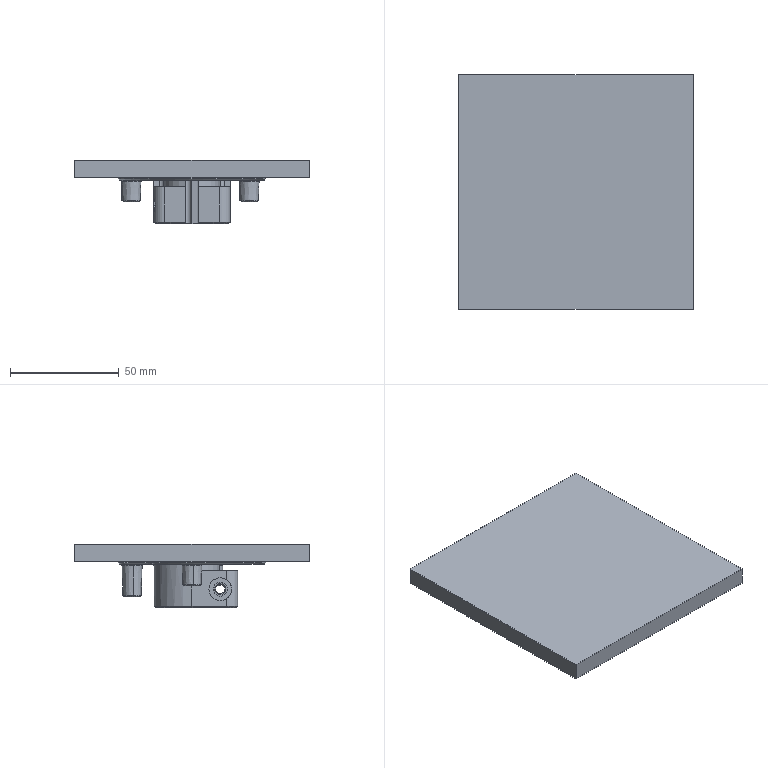NC program | NX | posted with a generic post | part box 108 x 108 x 29 mm
Lines 1354 to 2334 of 23883:
(CAVITY_MILL_COPY , TOOL : D6JING)
N2694 T16 M6
N2696 G54
N2698 G17 G0 G90 X1.893 Y-24.936 S9500 M3
N2700 G43 Z30. H16
N2702 Z1.115
N2704 G94 G1 Z-0.385 F1000.
N2706 X1.909 Y-24.321
N2708 G3 X1.432 Y-23.442 R1.
N2710 G2 X0. Y-20.885 R3. F1500.
N2712 G1 Y-20.5
N2714 Y-20.885
N2716 G2 X-1.432 Y-23.442 R3.
N2718 G3 X-1.909 Y-24.321 R1.
N2720 G1 X-1.893 Y-24.936
N2722 Z1.115
N2724 G0 Z30.
N2726 X1.893 Y-25.052
N2728 Z0.731
N2730 G1 Z-0.769 F1000.
N2732 X1.909 Y-24.437
N2734 G3 X1.432 Y-23.558 R1.
N2736 G2 X0. Y-21. R3. F1500.
N2738 G1 Y-20.5
N2740 Y-21.
N2742 G2 X-1.432 Y-23.558 R3.
N2744 G3 X-1.91 Y-24.437 R1.
N2746 G1 X-1.893 Y-25.052
N2748 Z0.731
N2750 G0 Z30.
N2752 X1.893
N2754 Z0.346
N2756 G1 Z-1.154 F1000.
N2758 X1.909 Y-24.437
N2760 G3 X1.432 Y-23.558 R1.
N2762 G2 X0. Y-21. R3. F1500.
N2764 G1 Y-20.5
N2766 Y-21.
N2768 G2 X-1.432 Y-23.558 R3.
N2770 G3 X-1.91 Y-24.437 R1.
N2772 G1 X-1.893 Y-25.052
N2774 Z0.346
N2776 G0 X1.893 Z-0.038
N2778 G1 Z-1.538 F1000.
N2780 X1.909 Y-24.437
N2782 G3 X1.432 Y-23.558 R1.
N2784 G2 X0. Y-21. R3. F1500.
N2786 G1 Y-20.5
N2788 Y-21.
N2790 G2 X-1.432 Y-23.558 R3.
N2792 G3 X-1.91 Y-24.437 R1.
N2794 G1 X-1.893 Y-25.052
N2796 Z-0.038
N2798 G0 X1.893 Z-0.423
N2800 G1 Z-1.923 F1000.
N2802 X1.909 Y-24.437
N2804 G3 X1.432 Y-23.558 R1.
N2806 G2 X0. Y-21. R3. F1500.
N2808 G1 Y-20.5
N2810 Y-21.
N2812 G2 X-1.432 Y-23.558 R3.
N2814 G3 X-1.91 Y-24.437 R1.
N2816 G1 X-1.893 Y-25.052
N2818 Z-0.423
N2820 G0 X1.893 Z-0.808
N2822 G1 Z-2.308 F1000.
N2824 X1.909 Y-24.437
N2826 G3 X1.432 Y-23.558 R1.
N2828 G2 X0. Y-21. R3. F1500.
N2830 G1 Y-20.5
N2832 Y-21.
N2834 G2 X-1.432 Y-23.558 R3.
N2836 G3 X-1.91 Y-24.437 R1.
N2838 G1 X-1.893 Y-25.052
N2840 Z-0.808
N2842 G0 X1.893 Z-1.192
N2844 G1 Z-2.692 F1000.
N2846 X1.909 Y-24.437
N2848 G3 X1.432 Y-23.558 R1.
N2850 G2 X0. Y-21. R3. F1500.
N2852 G1 Y-20.5
N2854 Y-21.
N2856 G2 X-1.432 Y-23.558 R3.
N2858 G3 X-1.91 Y-24.437 R1.
N2860 G1 X-1.893 Y-25.052
N2862 Z-1.192
N2864 G0 X1.893 Z-1.577
N2866 G1 Z-3.077 F1000.
N2868 X1.909 Y-24.437
N2870 G3 X1.432 Y-23.558 R1.
N2872 G2 X0. Y-21. R3. F1500.
N2874 G1 Y-20.5
N2876 Y-21.
N2878 G2 X-1.432 Y-23.558 R3.
N2880 G3 X-1.91 Y-24.437 R1.
N2882 G1 X-1.893 Y-25.052
N2884 Z-1.577
N2886 G0 X1.893 Z-1.962
N2888 G1 Z-3.462 F1000.
N2890 X1.909 Y-24.437
N2892 G3 X1.432 Y-23.558 R1.
N2894 G2 X0. Y-21. R3. F1500.
N2896 G1 Y-20.5
N2898 Y-21.
N2900 G2 X-1.432 Y-23.558 R3.
N2902 G3 X-1.91 Y-24.437 R1.
N2904 G1 X-1.893 Y-25.052
N2906 Z-1.962
N2908 G0 X1.893 Z-2.346
N2910 G1 Z-3.846 F1000.
N2912 X1.909 Y-24.437
N2914 G3 X1.432 Y-23.558 R1.
N2916 G2 X0. Y-21. R3. F1500.
N2918 G1 Y-20.5
N2920 Y-21.
N2922 G2 X-1.432 Y-23.558 R3.
N2924 G3 X-1.91 Y-24.437 R1.
N2926 G1 X-1.893 Y-25.052
N2928 Z-2.346
N2930 G0 X1.893 Z-2.731
N2932 G1 Z-4.231 F1000.
N2934 X1.909 Y-24.437
N2936 G3 X1.432 Y-23.558 R1.
N2938 G2 X0. Y-21. R3. F1500.
N2940 G1 Y-20.5
N2942 Y-21.
N2944 G2 X-1.432 Y-23.558 R3.
N2946 G3 X-1.91 Y-24.437 R1.
N2948 G1 X-1.893 Y-25.052
N2950 Z-2.731
N2952 G0 X1.893 Z-3.115
N2954 G1 Z-4.615 F1000.
N2956 X1.909 Y-24.437
N2958 G3 X1.432 Y-23.558 R1.
N2960 G2 X0. Y-21. R3. F1500.
N2962 G1 Y-20.501
N2964 Y-21.
N2966 G2 X-1.432 Y-23.558 R3.
N2968 G3 X-1.91 Y-24.437 R1.
N2970 G1 X-1.893 Y-25.052
N2972 Z-3.115
N2974 G0 X1.893 Z-3.5
N2976 G1 Z-5. F1000.
N2978 X1.909 Y-24.437
N2980 G3 X1.432 Y-23.558 R1.
N2982 G2 X0. Y-21. R3. F1500.
N2984 G1 Y-20.501
N2986 Y-21.
N2988 G2 X-1.432 Y-23.558 R3.
N2990 G3 X-1.91 Y-24.437 R1.
N2992 G1 X-1.893 Y-25.052
N2994 Z-3.5
N2996 G0 X1.893 Z-3.885
N2998 G1 Z-5.385 F1000.
N3000 X1.909 Y-24.437
N3002 G3 X1.432 Y-23.558 R1.
N3004 G2 X0. Y-21. R3. F1500.
N3006 G1 Y-20.501
N3008 Y-21.
N3010 G2 X-1.432 Y-23.558 R3.
N3012 G3 X-1.91 Y-24.437 R1.
N3014 G1 X-1.893 Y-25.052
N3016 Z-3.885
N3018 G0 X1.893 Z-4.269
N3020 G1 Z-5.769 F1000.
N3022 X1.909 Y-24.437
N3024 G3 X1.432 Y-23.558 R1.
N3026 G2 X0. Y-21. R3. F1500.
N3028 G1 Y-20.501
N3030 Y-21.
N3032 G2 X-1.432 Y-23.558 R3.
N3034 G3 X-1.91 Y-24.437 R1.
N3036 G1 X-1.893 Y-25.052
N3038 Z-4.269
N3040 G0 X1.893 Z-4.654
N3042 G1 Z-6.154 F1000.
N3044 X1.909 Y-24.437
N3046 G3 X1.432 Y-23.558 R1.
N3048 G2 X0. Y-21. R3. F1500.
N3050 G1 Y-20.501
N3052 Y-21.
N3054 G2 X-1.432 Y-23.558 R3.
N3056 G3 X-1.91 Y-24.437 R1.
N3058 G1 X-1.893 Y-25.052
N3060 Z-4.654
N3062 G0 X1.893 Z-5.038
N3064 G1 Z-6.538 F1000.
N3066 X1.909 Y-24.437
N3068 G3 X1.432 Y-23.558 R1.
N3070 G2 X0. Y-21. R3. F1500.
N3072 G1 Y-20.501
N3074 Y-21.
N3076 G2 X-1.432 Y-23.558 R3.
N3078 G3 X-1.91 Y-24.437 R1.
N3080 G1 X-1.893 Y-25.052
N3082 Z-5.038
N3084 G0 X1.893 Z-5.423
N3086 G1 Z-6.923 F1000.
N3088 X1.909 Y-24.437
N3090 G3 X1.432 Y-23.558 R1.
N3092 G2 X0. Y-21. R3. F1500.
N3094 G1 Y-20.501
N3096 Y-21.
N3098 G2 X-1.432 Y-23.558 R3.
N3100 G3 X-1.91 Y-24.437 R1.
N3102 G1 X-1.893 Y-25.052
N3104 Z-5.423
N3106 G0 X1.893 Z-5.808
N3108 G1 Z-7.308 F1000.
N3110 X1.909 Y-24.437
N3112 G3 X1.432 Y-23.558 R1.
N3114 G2 X0. Y-21. R3. F1500.
N3116 G1 Y-20.501
N3118 Y-21.
N3120 G2 X-1.432 Y-23.558 R3.
N3122 G3 X-1.91 Y-24.437 R1.
N3124 G1 X-1.893 Y-25.052
N3126 Z-5.808
N3128 G0 X1.893 Z-6.192
N3130 G1 Z-7.692 F1000.
N3132 X1.909 Y-24.437
N3134 G3 X1.432 Y-23.558 R1.
N3136 G2 X0. Y-21. R3. F1500.
N3138 G1 Y-20.501
N3140 Y-21.
N3142 G2 X-1.432 Y-23.558 R3.
N3144 G3 X-1.91 Y-24.437 R1.
N3146 G1 X-1.893 Y-25.052
N3148 Z-6.192
N3150 G0 X1.893 Z-6.577
N3152 G1 Z-8.077 F1000.
N3154 X1.909 Y-24.437
N3156 G3 X1.432 Y-23.558 R1.
N3158 G2 X0. Y-21. R3. F1500.
N3160 G1 Y-20.501
N3162 Y-21.
N3164 G2 X-1.432 Y-23.558 R3.
N3166 G3 X-1.91 Y-24.437 R1.
N3168 G1 X-1.893 Y-25.052
N3170 Z-6.577
N3172 G0 X1.893 Z-6.962
N3174 G1 Z-8.462 F1000.
N3176 X1.909 Y-24.437
N3178 G3 X1.432 Y-23.558 R1.
N3180 G2 X0. Y-21. R3. F1500.
N3182 G1 Y-20.501
N3184 Y-21.
N3186 G2 X-1.432 Y-23.558 R3.
N3188 G3 X-1.91 Y-24.437 R1.
N3190 G1 X-1.893 Y-25.052
N3192 Z-6.962
N3194 G0 X1.893 Z-7.346
N3196 G1 Z-8.846 F1000.
N3198 X1.909 Y-24.437
N3200 G3 X1.432 Y-23.558 R1.
N3202 G2 X0. Y-21. R3. F1500.
N3204 G1 Y-20.501
N3206 Y-21.
N3208 G2 X-1.432 Y-23.558 R3.
N3210 G3 X-1.91 Y-24.437 R1.
N3212 G1 X-1.893 Y-25.052
N3214 Z-7.346
N3216 G0 X1.893 Z-7.731
N3218 G1 Z-9.231 F1000.
N3220 X1.909 Y-24.437
N3222 G3 X1.432 Y-23.558 R1.
N3224 G2 X0. Y-21. R3. F1500.
N3226 G1 Y-20.501
N3228 Y-21.
N3230 G2 X-1.432 Y-23.558 R3.
N3232 G3 X-1.91 Y-24.437 R1.
N3234 G1 X-1.893 Y-25.052
N3236 Z-7.731
N3238 G0 X1.893 Z-8.115
N3240 G1 Z-9.615 F1000.
N3242 X1.909 Y-24.437
N3244 G3 X1.432 Y-23.558 R1.
N3246 G2 X0. Y-21. R3. F1500.
N3248 G1 Y-20.501
N3250 Y-21.
N3252 G2 X-1.432 Y-23.558 R3.
N3254 G3 X-1.91 Y-24.437 R1.
N3256 G1 X-1.893 Y-25.052
N3258 Z-8.115
N3260 G0 X1.893 Z-8.5
N3262 G1 Z-10. F1000.
N3264 X1.909 Y-24.437
N3266 G3 X1.432 Y-23.558 R1.
N3268 G2 X0. Y-21. R3. F1500.
N3270 G1 Y-20.501
N3272 Y-21.
N3274 G2 X-1.432 Y-23.558 R3.
N3276 G3 X-1.91 Y-24.437 R1.
N3278 G1 X-1.893 Y-25.052
N3280 Z-8.5
N3282 G0 X1.893 Z-8.9
N3284 G1 Z-10.4 F1000.
N3286 X1.909 Y-24.437
N3288 G3 X1.432 Y-23.558 R1.
N3290 G2 X0. Y-21. R3. F1500.
N3292 G1 Y-20.501
N3294 Y-21.
N3296 G2 X-1.432 Y-23.558 R3.
N3298 G3 X-1.91 Y-24.437 R1.
N3300 G1 X-1.893 Y-25.052
N3302 Z-8.9
N3304 G0 X1.893 Z-9.3
N3306 G1 Z-10.8 F1000.
N3308 X1.909 Y-24.437
N3310 G3 X1.432 Y-23.558 R1.
N3312 G2 X0. Y-21. R3. F1500.
N3314 G1 Y-20.501
N3316 Y-21.
N3318 G2 X-1.432 Y-23.558 R3.
N3320 G3 X-1.91 Y-24.437 R1.
N3322 G1 X-1.893 Y-25.052
N3324 Z-9.3
N3326 G0 X1.893 Z-9.7
N3328 G1 Z-11.2 F1000.
N3330 X1.909 Y-24.437
N3332 G3 X1.432 Y-23.558 R1.
N3334 G2 X0. Y-21. R3. F1500.
N3336 G1 Y-20.501
N3338 Y-21.
N3340 G2 X-1.432 Y-23.558 R3.
N3342 G3 X-1.91 Y-24.437 R1.
N3344 G1 X-1.893 Y-25.052
N3346 Z-9.7
N3348 G0 X1.893 Z-10.1
N3350 G1 Z-11.6 F1000.
N3352 X1.909 Y-24.437
N3354 G3 X1.432 Y-23.558 R1.
N3356 G2 X0. Y-21. R3. F1500.
N3358 G1 Y-20.501
N3360 Y-21.
N3362 G2 X-1.432 Y-23.558 R3.
N3364 G3 X-1.91 Y-24.437 R1.
N3366 G1 X-1.893 Y-25.052
N3368 Z-10.1
N3370 G0 X1.893 Z-10.5
N3372 G1 Z-12. F1000.
N3374 X1.909 Y-24.437
N3376 G3 X1.432 Y-23.558 R1.
N3378 G2 X0. Y-21. R3. F1500.
N3380 G1 Y-20.501
N3382 Y-21.
N3384 G2 X-1.432 Y-23.558 R3.
N3386 G3 X-1.91 Y-24.437 R1.
N3388 G1 X-1.893 Y-25.052
N3390 Z-10.5
N3392 G0 X1.893 Z-10.9
N3394 G1 Z-12.4 F1000.
N3396 X1.909 Y-24.437
N3398 G3 X1.432 Y-23.558 R1.
N3400 G2 X0. Y-21. R3. F1500.
N3402 G1 Y-20.501
N3404 Y-21.
N3406 G2 X-1.432 Y-23.558 R3.
N3408 G3 X-1.91 Y-24.437 R1.
N3410 G1 X-1.893 Y-25.052
N3412 Z-10.9
N3414 G0 X1.893 Z-11.3
N3416 G1 Z-12.8 F1000.
N3418 X1.909 Y-24.437
N3420 G3 X1.432 Y-23.558 R1.
N3422 G2 X0. Y-21. R3. F1500.
N3424 G1 Y-20.502
N3426 Y-21.
N3428 G2 X-1.432 Y-23.558 R3.
N3430 G3 X-1.91 Y-24.437 R1.
N3432 G1 X-1.893 Y-25.052
N3434 Z-11.3
N3436 G0 X1.893 Z-11.7
N3438 G1 Z-13.2 F1000.
N3440 X1.909 Y-24.437
N3442 G3 X1.432 Y-23.558 R1.
N3444 G2 X0. Y-21. R3. F1500.
N3446 G1 Y-20.502
N3448 Y-21.
N3450 G2 X-1.432 Y-23.558 R3.
N3452 G3 X-1.91 Y-24.437 R1.
N3454 G1 X-1.893 Y-25.052
N3456 Z-11.7
N3458 G0 X1.893 Z-12.1
N3460 G1 Z-13.6 F1000.
N3462 X1.909 Y-24.437
N3464 G3 X1.432 Y-23.558 R1.
N3466 G2 X0. Y-21. R3. F1500.
N3468 G1 Y-20.502
N3470 Y-21.
N3472 G2 X-1.432 Y-23.558 R3.
N3474 G3 X-1.91 Y-24.437 R1.
N3476 G1 X-1.893 Y-25.052
N3478 Z-12.1
N3480 G0 X1.893 Z-12.5
N3482 G1 Z-14. F1000.
N3484 X1.909 Y-24.437
N3486 G3 X1.432 Y-23.558 R1.
N3488 G2 X0. Y-21. R3. F1500.
N3490 G1 Y-20.502
N3492 Y-21.
N3494 G2 X-1.432 Y-23.558 R3.
N3496 G3 X-1.91 Y-24.437 R1.
N3498 G1 X-1.893 Y-25.052
N3500 Z-12.5
N3502 G0 X1.893 Z-12.9
N3504 G1 Z-14.4 F1000.
N3506 X1.909 Y-24.437
N3508 G3 X1.432 Y-23.558 R1.
N3510 G2 X0. Y-21. R3. F1500.
N3512 G1 Y-20.502
N3514 Y-21.
N3516 G2 X-1.432 Y-23.558 R3.
N3518 G3 X-1.91 Y-24.437 R1.
N3520 G1 X-1.893 Y-25.052
N3522 Z-12.9
N3524 G0 X1.893 Z-13.3
N3526 G1 Z-14.8 F1000.
N3528 X1.909 Y-24.437
N3530 G3 X1.432 Y-23.558 R1.
N3532 G2 X0. Y-21. R3. F1500.
N3534 G1 Y-20.502
N3536 Y-21.
N3538 G2 X-1.432 Y-23.558 R3.
N3540 G3 X-1.91 Y-24.437 R1.
N3542 G1 X-1.893 Y-25.052
N3544 Z-13.3
N3546 G0 X1.893 Z-13.7
N3548 G1 Z-15.2 F1000.
N3550 X1.909 Y-24.437
N3552 G3 X1.432 Y-23.558 R1.
N3554 G2 X0. Y-21. R3. F1500.
N3556 G1 Y-20.502
N3558 Y-21.
N3560 G2 X-1.432 Y-23.558 R3.
N3562 G3 X-1.91 Y-24.437 R1.
N3564 G1 X-1.893 Y-25.052
N3566 Z-13.7
N3568 G0 X1.893 Z-14.1
N3570 G1 Z-15.6 F1000.
N3572 X1.909 Y-24.437
N3574 G3 X1.432 Y-23.558 R1.
N3576 G2 X0. Y-21. R3. F1500.
N3578 G1 Y-20.502
N3580 Y-21.
N3582 G2 X-1.432 Y-23.558 R3.
N3584 G3 X-1.91 Y-24.437 R1.
N3586 G1 X-1.893 Y-25.052
N3588 Z-14.1
N3590 G0 X1.893 Z-14.5
N3592 G1 Z-16. F1000.
N3594 X1.909 Y-24.437
N3596 G3 X1.432 Y-23.558 R1.
N3598 G2 X0. Y-21. R3. F1500.
N3600 G1 Y-20.502
N3602 Y-21.
N3604 G2 X-1.432 Y-23.558 R3.
N3606 G3 X-1.91 Y-24.437 R1.
N3608 G1 X-1.893 Y-25.052
N3610 Z-14.5
N3612 G0 X1.893 Z-14.9
N3614 G1 Z-16.4 F1000.
N3616 X1.909 Y-24.437
N3618 G3 X1.432 Y-23.558 R1.
N3620 G2 X0. Y-21. R3. F1500.
N3622 G1 Y-20.502
N3624 Y-21.
N3626 G2 X-1.432 Y-23.558 R3.
N3628 G3 X-1.91 Y-24.437 R1.
N3630 G1 X-1.893 Y-25.052
N3632 Z-14.9
N3634 G0 X1.893 Z-15.3
N3636 G1 Z-16.8 F1000.
N3638 X1.909 Y-24.437
N3640 G3 X1.432 Y-23.558 R1.
N3642 G2 X0. Y-21. R3. F1500.
N3644 G1 Y-20.502
N3646 Y-21.
N3648 G2 X-1.432 Y-23.558 R3.
N3650 G3 X-1.91 Y-24.437 R1.
N3652 G1 X-1.893 Y-25.052
N3654 Z-15.3
N3656 G0 X1.893 Z-15.7
N3658 G1 Z-17.2 F1000.
N3660 X1.909 Y-24.437
N3662 G3 X1.432 Y-23.558 R1.
N3664 G2 X0.009 Y-21.23 R3. F1500.
N3666 G1 X-0.012 Y-21.232
N3668 X-0.011 Y-21.253
N3670 G2 X-1.432 Y-23.558 R3.
N3672 G3 X-1.909 Y-24.437 R1.
N3674 G1 X-1.893 Y-25.052
N3676 Z-15.7
N3678 G0 X1.893 Z-16.1
N3680 G1 Z-17.6 F1000.
N3682 X1.909 Y-24.437
N3684 G3 X1.432 Y-23.558 R1.
N3686 G2 X0.009 Y-21.23 R3. F1500.
N3688 G1 X-0.012 Y-21.232
N3690 X-0.011 Y-21.253
N3692 G2 X-1.432 Y-23.558 R3.
N3694 G3 X-1.909 Y-24.437 R1.
N3696 G1 X-1.893 Y-25.052
N3698 Z-16.1
N3700 G0 X1.893 Z-16.5
N3702 G1 Z-18. F1000.
N3704 X1.909 Y-24.437
N3706 G3 X1.432 Y-23.558 R1.
N3708 G2 X0.009 Y-21.23 R3. F1500.
N3710 G1 X-0.012 Y-21.232
N3712 X-0.011 Y-21.253
N3714 G2 X-1.432 Y-23.558 R3.
N3716 G3 X-1.909 Y-24.437 R1.
N3718 G1 X-1.893 Y-25.052
N3720 Z-16.5
N3722 G0 X1.893 Z-16.9
N3724 G1 Z-18.4 F1000.
N3726 X1.909 Y-24.437
N3728 G3 X1.432 Y-23.558 R1.
N3730 G2 X0.009 Y-21.23 R3. F1500.
N3732 G1 X-0.012 Y-21.232
N3734 X-0.011 Y-21.253
N3736 G2 X-1.432 Y-23.558 R3.
N3738 G3 X-1.909 Y-24.437 R1.
N3740 G1 X-1.893 Y-25.052
N3742 Z-16.9
N3744 G0 X1.893 Z-17.3
N3746 G1 Z-18.8 F1000.
N3748 X1.909 Y-24.437
N3750 G3 X1.432 Y-23.558 R1.
N3752 G2 X0.009 Y-21.23 R3. F1500.
N3754 G1 X-0.012 Y-21.232
N3756 X-0.011 Y-21.253
N3758 G2 X-1.432 Y-23.558 R3.
N3760 G3 X-1.909 Y-24.437 R1.
N3762 G1 X-1.893 Y-25.052
N3764 Z-17.3
N3766 G0 X1.893 Z-17.7
N3768 G1 Z-19.2 F1000.
N3770 X1.91 Y-24.437
N3772 G3 X1.432 Y-23.558 R1.
N3774 G2 X0.009 Y-21.23 R3. F1500.
N3776 G1 X-0.012 Y-21.232
N3778 X-0.011 Y-21.253
N3780 G2 X-1.432 Y-23.558 R3.
N3782 G3 X-1.91 Y-24.437 R1.
N3784 G1 X-1.893 Y-25.052
N3786 Z-17.7
N3788 G0 X1.893 Z-18.1
N3790 G1 Z-19.6 F1000.
N3792 X1.909 Y-24.437
N3794 G3 X1.432 Y-23.558 R1.
N3796 G2 X0.009 Y-21.23 R3. F1500.
N3798 G1 X-0.012 Y-21.232
N3800 X-0.011 Y-21.254
N3802 G2 X-1.432 Y-23.558 R3.
N3804 G3 X-1.909 Y-24.437 R1.
N3806 G1 X-1.893 Y-25.052
N3808 Z-18.1
N3810 G0 X1.894 Z-18.5
N3812 G1 Z-20. F1000.
N3814 X1.91 Y-24.437
N3816 G3 X1.433 Y-23.558 R1.
N3818 G2 X0.009 Y-21.23 R3. F1500.
N3820 G1 X-0.012 Y-21.232
N3822 X-0.011 Y-21.254
N3824 G2 X-1.433 Y-23.558 R3.
N3826 G3 X-1.91 Y-24.437 R1.
N3828 G1 X-1.894 Y-25.052
N3830 Z-18.5
N3832 G0 Z30.
N3834 X-21.148 Y-19.14
N3836 Z-8.9
N3838 G1 Z-10.4 F1000.
N3840 X-20.62 Y-18.659
N3842 G3 X-20.316 Y-17.706 R1.
N3844 G2 X-20.5 Y-16. R8. F1500.
N3846 G1 Y-13.766
N3848 G2 X-23.426 Y-16.134 R7.164
N3850 G3 X-24.017 Y-16.941 R1.
N3852 G1 X-24.094 Y-17.642
N3854 Z-8.9
N3856 G0 X-21.11 Y-19.241 Z-9.3
N3858 G1 Z-10.8 F1000.
N3860 X-20.588 Y-18.755
N3862 G3 X-20.295 Y-17.798 R1.
N3864 G2 X-20.5 Y-16. R8. F1500.
N3866 G1 Y-13.958
N3868 G2 X-23.398 Y-16.246 R7.278
N3870 G3 X-23.991 Y-17.051 R1.
N3872 G1 X-24.07 Y-17.753
N3874 Z-9.3
N3876 G0 X-21.105 Y-19.254 Z-9.7
N3878 G1 Z-11.2 F1000.
N3880 X-20.584 Y-18.766
N3882 G3 X-20.293 Y-17.81 R1.
N3884 G2 X-20.5 Y-16. R8. F1500.
N3886 G1 Y-13.981
N3888 G2 X-23.394 Y-16.26 R7.292
N3890 G3 X-23.988 Y-17.064 R1.
N3892 G1 X-24.067 Y-17.767
N3894 Z-9.7
N3896 G0 X-21.101 Y-19.266 Z-10.1
N3898 G1 Z-11.6 F1000.
N3900 X-20.58 Y-18.778
N3902 G3 X-20.29 Y-17.821 R1.
N3904 G2 X-20.5 Y-16. R8. F1500.
N3906 G1 Y-14.004
N3908 G2 X-23.391 Y-16.273 R7.306
N3910 G3 X-23.985 Y-17.078 R1.
N3912 G1 X-24.064 Y-17.78
N3914 Z-10.1
N3916 G0 X-21.096 Y-19.279 Z-10.5
N3918 G1 Z-12. F1000.
N3920 X-20.576 Y-18.789
N3922 G3 X-20.287 Y-17.832 R1.
N3924 G2 X-20.5 Y-16. R8. F1500.
N3926 G1 Y-14.027
N3928 G2 X-23.387 Y-16.287 R7.32
N3930 G3 X-23.982 Y-17.091 R1.
N3932 G1 X-24.061 Y-17.794
N3934 Z-10.5
N3936 G0 X-21.091 Y-19.291 Z-10.9
N3938 G1 Z-12.4 F1000.
N3940 X-20.572 Y-18.801
N3942 G3 X-20.285 Y-17.843 R1.
N3944 G2 X-20.5 Y-16. R8. F1500.
N3946 G1 Y-14.05
N3948 G2 X-23.384 Y-16.301 R7.334
N3950 G3 X-23.978 Y-17.105 R1.
N3952 G1 X-24.058 Y-17.807
N3954 Z-10.9
N3956 G0 X-21.087 Y-19.303 Z-11.3
N3958 G1 Z-12.8 F1000.
N3960 X-20.568 Y-18.813
N3962 G3 X-20.282 Y-17.854 R1.
N3964 G2 X-20.5 Y-16. R8. F1500.
N3966 G1 Y-14.073
N3968 G2 X-23.38 Y-16.314 R7.348
N3970 G3 X-23.975 Y-17.118 R1.
N3972 G1 X-24.055 Y-17.821
N3974 Z-11.3
N3976 G0 X-21.082 Y-19.316 Z-11.7
N3978 G1 Z-13.2 F1000.
N3980 X-20.564 Y-18.824
N3982 G3 X-20.279 Y-17.866 R1.
N3984 G2 X-20.5 Y-16. R8. F1500.
N3986 G1 Y-14.096
N3988 G2 X-23.377 Y-16.328 R7.362
N3990 G3 X-23.972 Y-17.132 R1.
N3992 G1 X-24.052 Y-17.835
N3994 Z-11.7
N3996 G0 X-21.077 Y-19.328 Z-12.1
N3998 G1 Z-13.6 F1000.
N4000 X-20.56 Y-18.836
N4002 G3 X-20.277 Y-17.877 R1.
N4004 G2 X-20.5 Y-16. R8. F1500.
N4006 G1 Y-14.118
N4008 G2 X-23.373 Y-16.342 R7.376
N4010 G3 X-23.968 Y-17.145 R1.
N4012 G1 X-24.049 Y-17.848
N4014 Z-12.1
N4016 G0 X-21.072 Y-19.34 Z-12.5
N4018 G1 Z-14. F1000.
N4020 X-20.556 Y-18.847
N4022 G3 X-20.274 Y-17.888 R1.
N4024 G2 X-20.5 Y-16. R8. F1500.
N4026 G1 Y-14.141
N4028 G2 X-23.369 Y-16.355 R7.39
N4030 G3 X-23.965 Y-17.159 R1.
N4032 G1 X-24.045 Y-17.862
N4034 Z-12.5
N4036 G0 X-21.067 Y-19.353 Z-12.9
N4038 G1 Z-14.4 F1000.
N4040 X-20.551 Y-18.859
N4042 G3 X-20.271 Y-17.899 R1.
N4044 G2 X-20.5 Y-16. R8. F1500.
N4046 G1 Y-14.164
N4048 G2 X-23.366 Y-16.369 R7.404
N4050 G3 X-23.961 Y-17.172 R1.
N4052 G1 X-24.042 Y-17.876
N4054 Z-12.9
N4056 G0 X-21.063 Y-19.365 Z-13.3
N4058 G1 Z-14.8 F1000.
N4060 X-20.547 Y-18.871
N4062 G3 X-20.269 Y-17.91 R1.
N4064 G2 X-20.5 Y-16. R8. F1500.
N4066 G1 Y-14.186
N4068 G2 X-23.362 Y-16.383 R7.418
N4070 G3 X-23.958 Y-17.186 R1.
N4072 G1 X-24.039 Y-17.889
N4074 Z-13.3
N4076 G0 X-21.058 Y-19.377 Z-13.7
N4078 G1 Z-15.2 F1000.
N4080 X-20.543 Y-18.882
N4082 G3 X-20.266 Y-17.921 R1.
N4084 G2 X-20.5 Y-16. R8. F1500.
N4086 G1 Y-14.209
N4088 G2 X-23.358 Y-16.396 R7.432
N4090 G3 X-23.955 Y-17.199 R1.
N4092 G1 X-24.036 Y-17.903
N4094 Z-13.7
N4096 G0 X-21.05 Y-19.396 Z-14.1
N4098 G1 Z-15.6 F1000.
N4100 X-20.537 Y-18.899
N4102 G3 X-20.262 Y-17.938 R1.
N4104 G2 X-20.5 Y-16. R8. F1500.
N4106 G1 Y-14.231
N4108 G2 X-23.355 Y-16.41 R7.446
N4110 G3 X-23.952 Y-17.213 R1.
N4112 G1 X-24.033 Y-17.917
N4114 Z-14.1
N4116 G0 X-21.046 Y-19.407 Z-14.5
N4118 G1 Z-16. F1000.
N4120 X-20.533 Y-18.91
N4122 G3 X-20.259 Y-17.948 R1.
N4124 G2 X-20.5 Y-16. R8. F1500.
N4126 G1 Y-14.253
N4128 G2 X-23.352 Y-16.424 R7.46
N4130 G3 X-23.948 Y-17.226 R1.
N4132 G1 X-24.03 Y-17.93
N4134 Z-14.5
N4136 G0 X-21.042 Y-19.418 Z-14.9
N4138 G1 Z-16.4 F1000.
N4140 X-20.529 Y-18.92
N4142 G3 X-20.257 Y-17.958 R1.
N4144 G2 X-20.5 Y-16. R8. F1500.
N4146 G1 Y-14.276
N4148 G2 X-23.348 Y-16.437 R7.473
N4150 G3 X-23.945 Y-17.24 R1.
N4152 G1 X-24.027 Y-17.944
N4154 Z-14.9
N4156 G0 X-21.037 Y-19.429 Z-15.3
N4158 G1 Z-16.8 F1000.
N4160 X-20.526 Y-18.931
N4162 G3 X-20.254 Y-17.968 R1.
N4164 G2 X-20.5 Y-16. R8. F1500.
N4166 G1 Y-14.298
N4168 G2 X-23.344 Y-16.451 R7.487
N4170 G3 X-23.941 Y-17.253 R1.
N4172 G1 X-24.023 Y-17.957
N4174 Z-15.3
N4176 G0 X-21.033 Y-19.44 Z-15.7
N4178 G1 Z-17.2 F1000.
N4180 X-20.522 Y-18.942
N4182 G3 X-20.251 Y-17.979 R1.
N4184 G2 X-20.5 Y-16. R8. F1500.
N4186 G1 Y-14.32
N4188 G2 X-23.34 Y-16.465 R7.501
N4190 G3 X-23.937 Y-17.267 R1.
N4192 G1 X-24.02 Y-17.971
N4194 Z-15.7
N4196 G0 X-21.028 Y-19.452 Z-16.1
N4198 G1 Z-17.6 F1000.
N4200 X-20.518 Y-18.952
N4202 G3 X-20.249 Y-17.989 R1.
N4204 G2 X-20.5 Y-16. R8. F1500.
N4206 G1 Y-14.342
N4208 G2 X-23.336 Y-16.478 R7.515
N4210 G3 X-23.934 Y-17.28 R1.
N4212 G1 X-24.016 Y-17.984
N4214 Z-16.1
N4216 G0 X-21.023 Y-19.464 Z-16.5
N4218 G1 Z-18. F1000.
N4220 X-20.514 Y-18.964
N4222 G3 X-20.246 Y-18. R1.
N4224 G2 X-20.5 Y-16. R8. F1500.
N4226 G1 Y-14.364
N4228 G2 X-23.333 Y-16.492 R7.529
N4230 G3 X-23.93 Y-17.293 R1.
N4232 G1 X-24.013 Y-17.998
N4234 Z-16.5
N4236 G0 X-21.018 Y-19.476 Z-16.9
N4238 G1 Z-18.4 F1000.
N4240 X-20.509 Y-18.975
N4242 G3 X-20.243 Y-18.011 R1.
N4244 G2 X-20.5 Y-16. R8. F1500.
N4246 G1 Y-14.386
N4248 G2 X-23.329 Y-16.505 R7.543
N4250 G3 X-23.927 Y-17.307 R1.
N4252 G1 X-24.01 Y-18.011
N4254 Z-16.9
N4256 G0 X-21.013 Y-19.488 Z-17.3
N4258 G1 Z-18.8 F1000.
N4260 X-20.505 Y-18.986
N4262 G3 X-20.24 Y-18.022 R1.
N4264 G2 X-20.5 Y-16. R8. F1500.
N4266 G1 Y-14.408
N4268 G2 X-23.325 Y-16.519 R7.557
N4270 G3 X-23.923 Y-17.32 R1.
N4272 G1 X-24.006 Y-18.025
N4274 Z-17.3
N4276 G0 X-21.008 Y-19.5 Z-17.7
N4278 G1 Z-19.2 F1000.
N4280 X-20.501 Y-18.998
N4282 G3 X-20.237 Y-18.033 R1.
N4284 G2 X-20.5 Y-16. R8. F1500.
N4286 G1 Y-14.43
N4288 G2 X-23.321 Y-16.532 R7.571
N4290 G3 X-23.92 Y-17.334 R1.
N4292 G1 X-24.003 Y-18.039
N4294 Z-17.7
N4296 G0 X-20.976 Y-19.577 Z-18.1
N4298 G1 Z-19.6 F1000.
N4300 X-20.474 Y-19.07
N4302 G3 X-20.219 Y-18.103 R1.
N4304 G2 X-20.5 Y-16. R8. F1500.
N4306 G1 Y-14.567
N4308 G2 X-23.297 Y-16.619 R7.66
N4310 G3 X-23.896 Y-17.419 R1.
N4312 G1 X-23.981 Y-18.125
N4314 Z-18.1
N4316 G0 X-20.741 Y-20.089 Z-18.5
N4318 G1 Z-20. F1000.
N4320 X-20.271 Y-19.552
N4322 G3 X-20.076 Y-18.571 R1.
N4324 G2 X-20.5 Y-16. R8. F1500.
N4326 G1 Y-15.45
N4328 G2 X-23.117 Y-17.197 R8.262
N4330 G3 X-23.723 Y-17.992 R1.
N4332 G1 X-23.813 Y-18.703
N4334 Z-18.5
N4336 G0 Z30.
N4338 X-24.259 Y-1.468
N4340 Z-8.9
N4342 G1 Z-10.4 F1000.
N4344 X-24.168 Y-2.167
N4346 G3 X-23.56 Y-2.962 R1.
N4348 G2 X-20.5 Y-5.387 R7.164 F1500.
N4350 G1 Y-1.026
N4352 G3 X-21. Y-0.16 R1.
N4354 G1 X-21.699 Y0.243
N4356 Z-8.9
N4358 G0 X-24.257 Y-1.351 Z-9.3
N4360 G1 Z-10.8 F1000.
N4362 X-24.162 Y-2.052
N4364 G3 X-23.55 Y-2.843 R1.
N4366 G2 X-20.5 Y-5.195 R7.278 F1500.
N4368 G1 Y-0.901
N4370 G3 X-21. Y-0.035 R1.
N4372 G1 X-21.697 Y0.367
N4374 Z-9.3
N4376 G0 X-24.256 Y-1.337 Z-9.7
N4378 G1 Z-11.2 F1000.
N4380 X-24.161 Y-2.037
N4382 G3 X-23.549 Y-2.828 R1.
N4384 G2 X-20.5 Y-5.172 R7.292 F1500.
N4386 G1 Y-0.886
N4388 G3 X-21. Y-0.02 R1.
N4390 G1 X-21.697 Y0.382
N4392 Z-9.7
N4394 G0 X-24.256 Y-1.323 Z-10.1
N4396 G1 Z-11.6 F1000.
N4398 X-24.16 Y-2.023
N4400 G3 X-23.548 Y-2.814 R1.
N4402 G2 X-20.5 Y-5.149 R7.306 F1500.
N4404 G1 Y-0.871
N4406 G3 X-21. Y-0.005 R1.
N4408 G1 X-21.696 Y0.398
N4410 Z-10.1
N4412 G0 X-24.256 Y-1.308 Z-10.5
N4414 G1 Z-12. F1000.
N4416 X-24.16 Y-2.009
N4418 G3 X-23.547 Y-2.799 R1.
N4420 G2 X-20.5 Y-5.126 R7.32 F1500.
N4422 G1 Y-0.855
N4424 G3 X-21. Y0.011 R1.
N4426 G1 X-21.696 Y0.413
N4428 Z-10.5
N4430 G0 X-24.255 Y-1.294 Z-10.9
N4432 G1 Z-12.4 F1000.
N4434 X-24.159 Y-1.995
N4436 G3 X-23.545 Y-2.784 R1.
N4438 G2 X-20.5 Y-5.103 R7.334 F1500.
N4440 G1 Y-0.84
N4442 G3 X-21. Y0.026 R1.
N4444 G1 X-21.696 Y0.428
N4446 Z-10.9
N4448 G0 X-24.255 Y-1.28 Z-11.3
N4450 G1 Z-12.8 F1000.
N4452 X-24.158 Y-1.98
N4454 G3 X-23.544 Y-2.77 R1.
N4456 G2 X-20.5 Y-5.08 R7.348 F1500.
N4458 G1 Y-0.825
N4460 G3 X-21. Y0.041 R1.
N4462 G1 X-21.695 Y0.443
N4464 Z-11.3
N4466 G0 X-24.255 Y-1.265 Z-11.7
N4468 G1 Z-13.2 F1000.
N4470 X-24.157 Y-1.966
N4472 G3 X-23.543 Y-2.755 R1.
N4474 G2 X-20.5 Y-5.057 R7.362 F1500.
N4476 G1 Y-0.809
N4478 G3 X-21. Y0.057 R1.
N4480 G1 X-21.695 Y0.458
N4482 Z-11.7
N4484 G0 X-24.255 Y-1.251 Z-12.1
N4486 G1 Z-13.6 F1000.
N4488 X-24.157 Y-1.952
N4490 G3 X-23.542 Y-2.741 R1.
N4492 G2 X-20.5 Y-5.035 R7.376 F1500.
N4494 G1 Y-0.794
N4496 G3 X-21. Y0.072 R1.
N4498 G1 X-21.695 Y0.473
N4500 Z-12.1
N4502 G0 X-24.254 Y-1.237 Z-12.5
N4504 G1 Z-14. F1000.
N4506 X-24.156 Y-1.938
N4508 G3 X-23.541 Y-2.726 R1.
N4510 G2 X-20.5 Y-5.012 R7.39 F1500.
N4512 G1 Y-0.779
N4514 G3 X-21. Y0.087 R1.
N4516 G1 X-21.695 Y0.488
N4518 Z-12.5
N4520 G0 X-24.254 Y-1.223 Z-12.9
N4522 G1 Z-14.4 F1000.
N4524 X-24.155 Y-1.924
N4526 G3 X-23.539 Y-2.711 R1.
N4528 G2 X-20.5 Y-4.989 R7.404 F1500.
N4530 G1 Y-0.763
N4532 G3 X-21. Y0.103 R1.
N4534 G1 X-21.694 Y0.503
N4536 Z-12.9
N4538 G0 X-24.254 Y-1.208 Z-13.3
N4540 G1 Z-14.8 F1000.
N4542 X-24.155 Y-1.909
N4544 G3 X-23.538 Y-2.697 R1.
N4546 G2 X-20.5 Y-4.967 R7.418 F1500.
N4548 G1 Y-0.748
N4550 G3 X-21. Y0.118 R1.
N4552 G1 X-21.694 Y0.518
N4554 Z-13.3
N4556 G0 X-24.253 Y-1.194 Z-13.7
N4558 G1 Z-15.2 F1000.
N4560 X-24.154 Y-1.895
N4562 G3 X-23.537 Y-2.682 R1.
N4564 G2 X-20.5 Y-4.944 R7.432 F1500.
N4566 G1 Y-0.733
N4568 G3 X-21. Y0.133 R1.
N4570 G1 X-21.693 Y0.533
N4572 Z-13.7
N4574 G0 X-24.253 Y-1.18 Z-14.1
N4576 G1 Z-15.6 F1000.
N4578 X-24.153 Y-1.881
N4580 G3 X-23.536 Y-2.668 R1.
N4582 G2 X-20.5 Y-4.922 R7.446 F1500.
N4584 G1 Y-0.718
N4586 G3 X-21. Y0.148 R1.
N4588 G1 X-21.693 Y0.548
N4590 Z-14.1
N4592 G0 X-24.253 Y-1.165 Z-14.5
N4594 G1 Z-16. F1000.
N4596 X-24.152 Y-1.867
N4598 G3 X-23.535 Y-2.653 R1.
N4600 G2 X-20.5 Y-4.9 R7.46 F1500.
N4602 G1 Y-0.702
N4604 G3 X-21. Y0.164 R1.
N4606 G1 X-21.693 Y0.564
N4608 Z-14.5
N4610 G0 X-24.252 Y-1.151 Z-14.9
N4612 G1 Z-16.4 F1000.
N4614 X-24.152 Y-1.852
N4616 G3 X-23.534 Y-2.639 R1.
N4618 G2 X-20.5 Y-4.878 R7.473 F1500.
N4620 G1 Y-0.687
N4622 G3 X-21. Y0.179 R1.
N4624 G1 X-21.692 Y0.579
N4626 Z-14.9
N4628 G0 X-24.252 Y-1.137 Z-15.3
N4630 G1 Z-16.8 F1000.
N4632 X-24.151 Y-1.838
N4634 G3 X-23.532 Y-2.624 R1.
N4636 G2 X-20.5 Y-4.855 R7.487 F1500.
N4638 G1 Y-0.672
N4640 G3 X-21. Y0.194 R1.
N4642 G1 X-21.692 Y0.594
N4644 Z-15.3
N4646 G0 X-24.252 Y-1.122 Z-15.7
N4648 G1 Z-17.2 F1000.